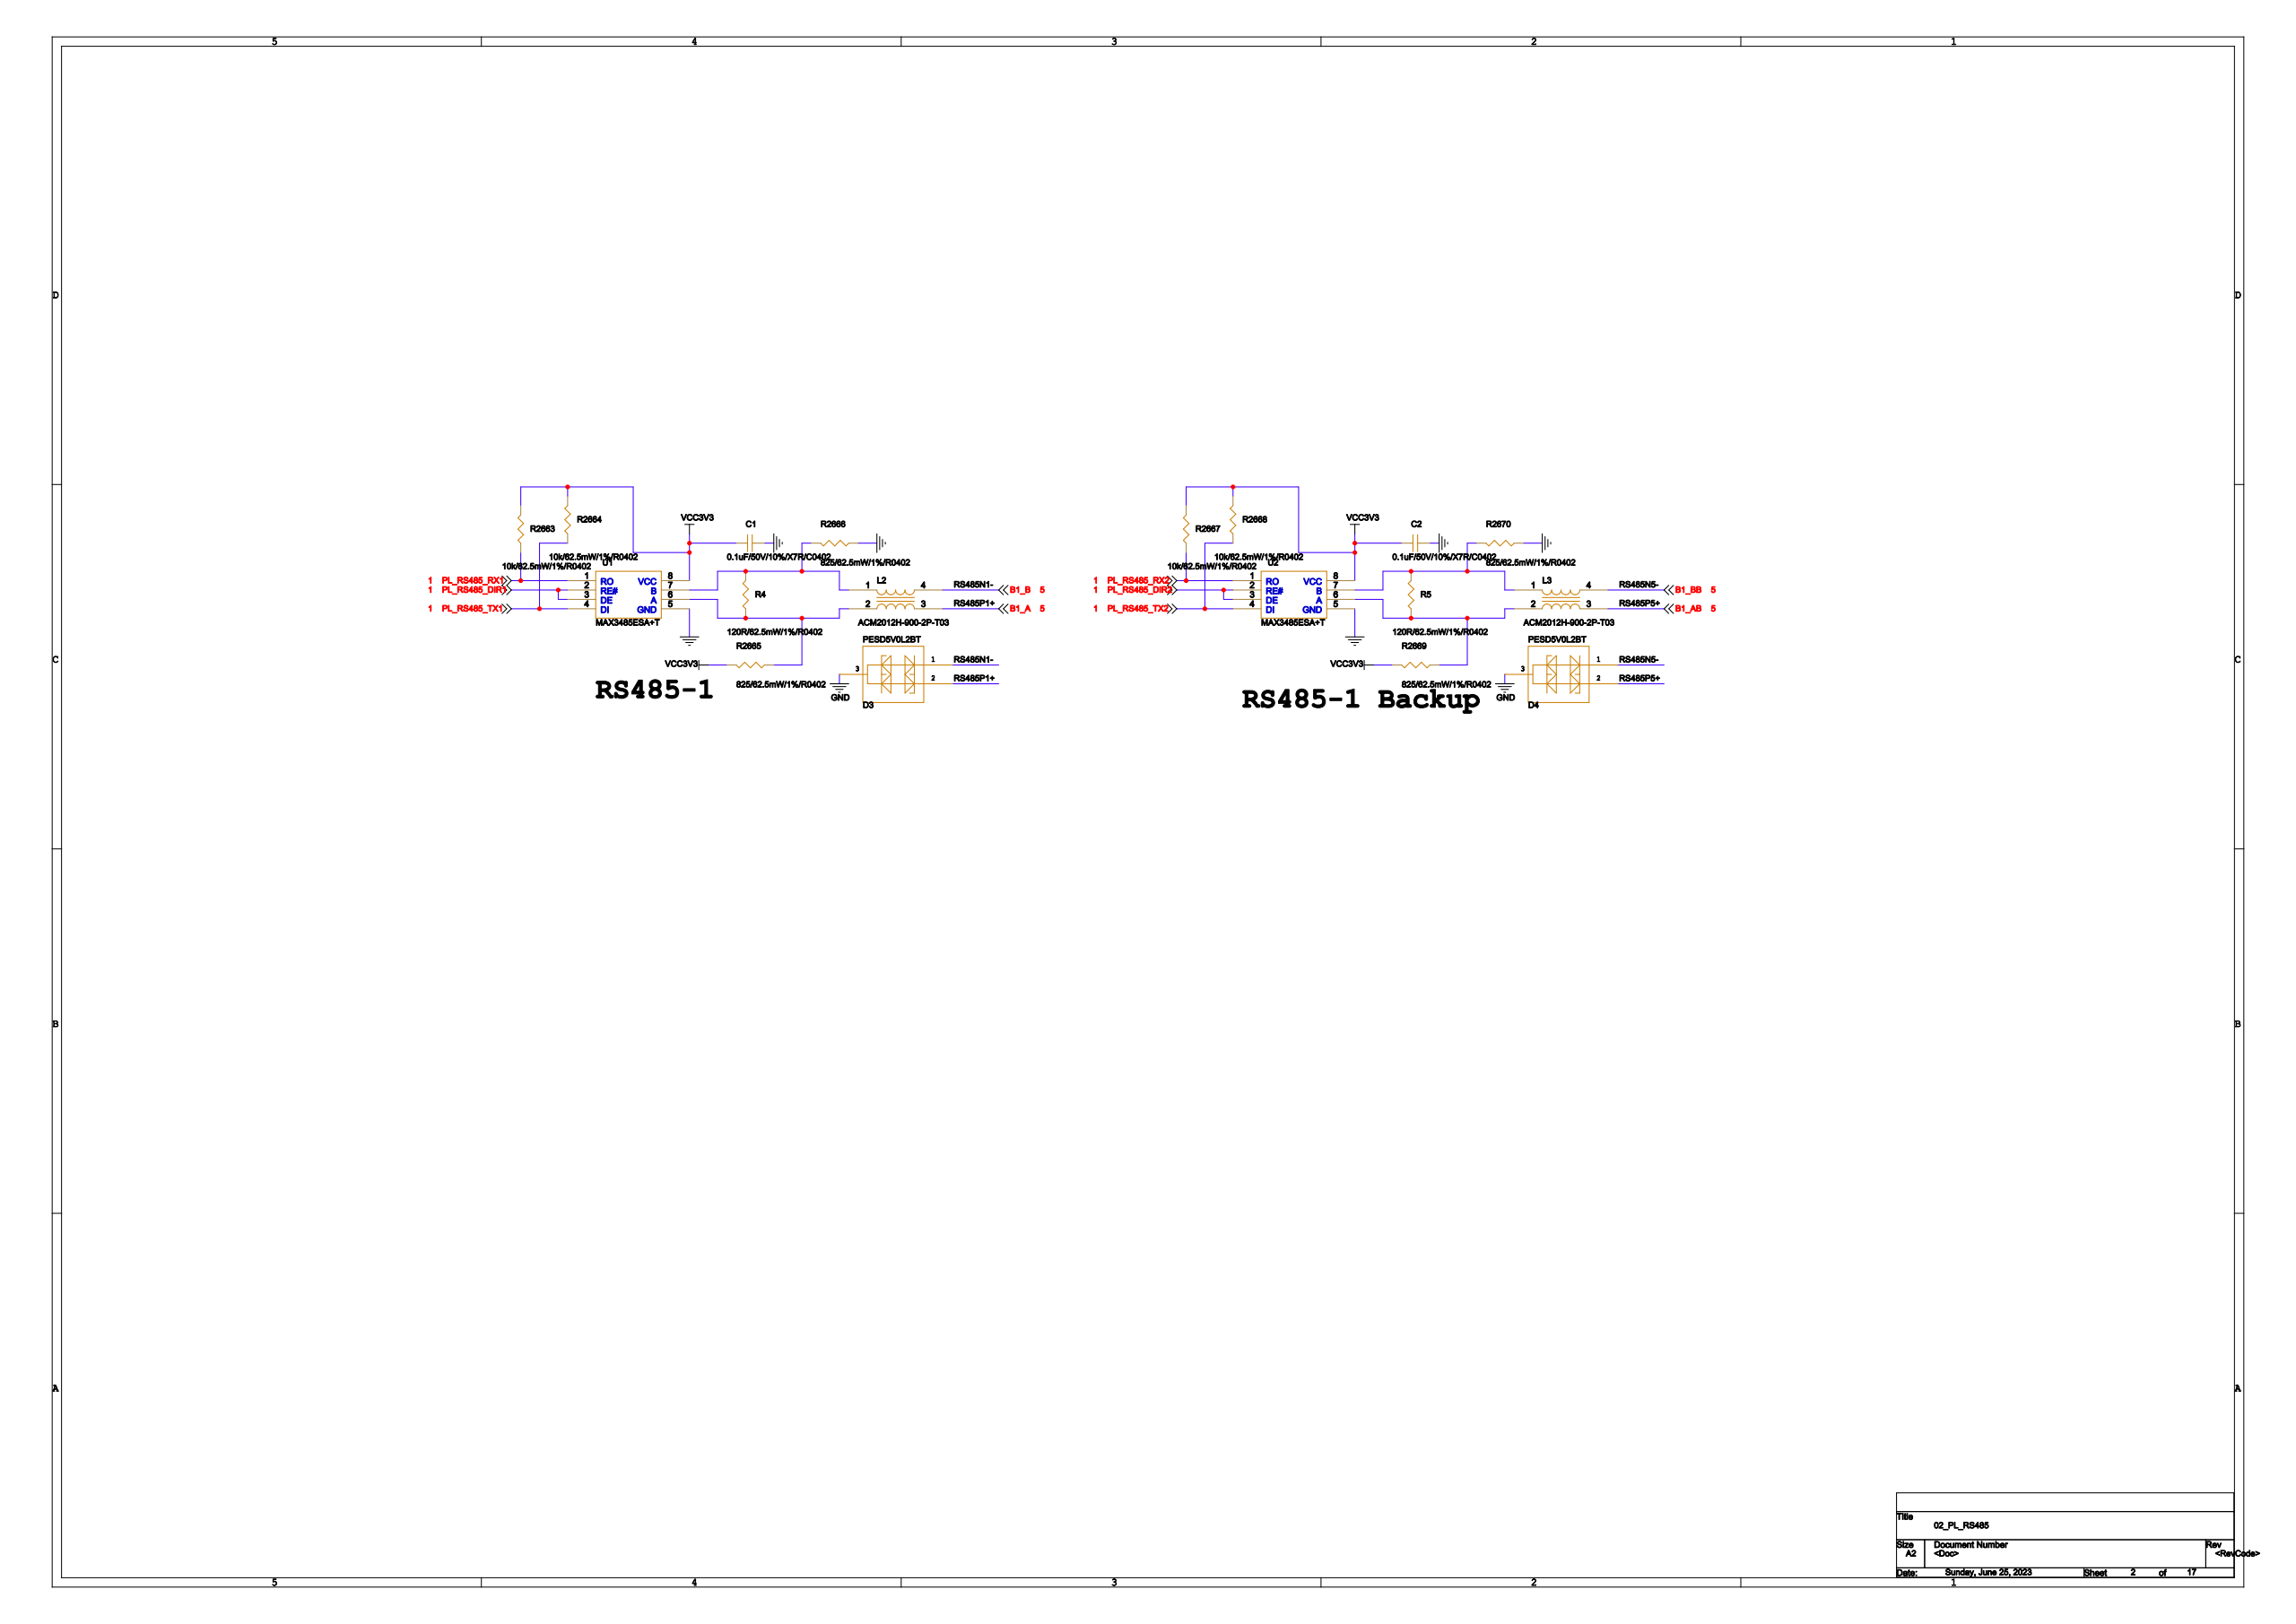Circuit board | Cadence Allegro | 1997 parts | 1536 nets | one sheet of the schematic
Parts on this sheet (reference | value | footprint):
C1 | 0.1uF/50V/10%/X7R/C0402 | 0402
C2 | 0.1uF/50V/10%/X7R/C0402 | 0402
D3 | PESD5V0L2BT | SOT23
D4 | PESD5V0L2BT | SOT23
L2 | ACM2012H-900-2P-T03 | ACM2012
L3 | ACM2012H-900-2P-T03 | ACM2012
R4 | 120R/62.5mW/1%/R0402 | 0402
R5 | 120R/62.5mW/1%/R0402 | 0402
R2663 | 10K/62.5mW/1%/R0402 | 0402
R2664 | 10K/62.5mW/1%/R0402 | 0402
R2665 | 825/62.5mW/1%/R0402 | 0402
R2666 | 825/62.5mW/1%/R0402 | 0402
R2667 | 10K/62.5mW/1%/R0402 | 0402
R2668 | 10K/62.5mW/1%/R0402 | 0402
R2669 | 825/62.5mW/1%/R0402 | 0402
R2670 | 825/62.5mW/1%/R0402 | 0402
U1 | MAX3485ESA+T | SO8
U2 | MAX3485ESA+T | SO8
Nets of these parts (net: part-pin ...):
3.3V: C1-1 C2-1 R2663-1 R2664-1 R2665-1 R2667-1 R2668-1 R2669-1 U1-8 U2-8
N21786216: L2-2 R4-2 R2665-2 U1-6
N21786207: L2-1 R4-1 R2666-1 U1-7
AGND: C1-2 C2-2 D3-3 D4-3 R2666-2 R2670-2 U1-5 U2-5
N23300015: L3-2 R5-2 R2669-2 U2-6
N23300009: L3-1 R5-1 R2670-1 U2-7
PL_RS485_TX1: R2664-2 U1-4
PL_RS485_DIR1: U1-2 U1-3
PL_RS485_RX1: R2663-2 U1-1
PL_RS485_TX2: R2668-2 U2-4
PL_RS485_DIR2: U2-2 U2-3
PL_RS485_RX2: R2667-2 U2-1
B1_A: D3-2 L2-3
B1_B: D3-1 L2-4
B1_AB: D4-2 L3-3
B1_BB: D4-1 L3-4